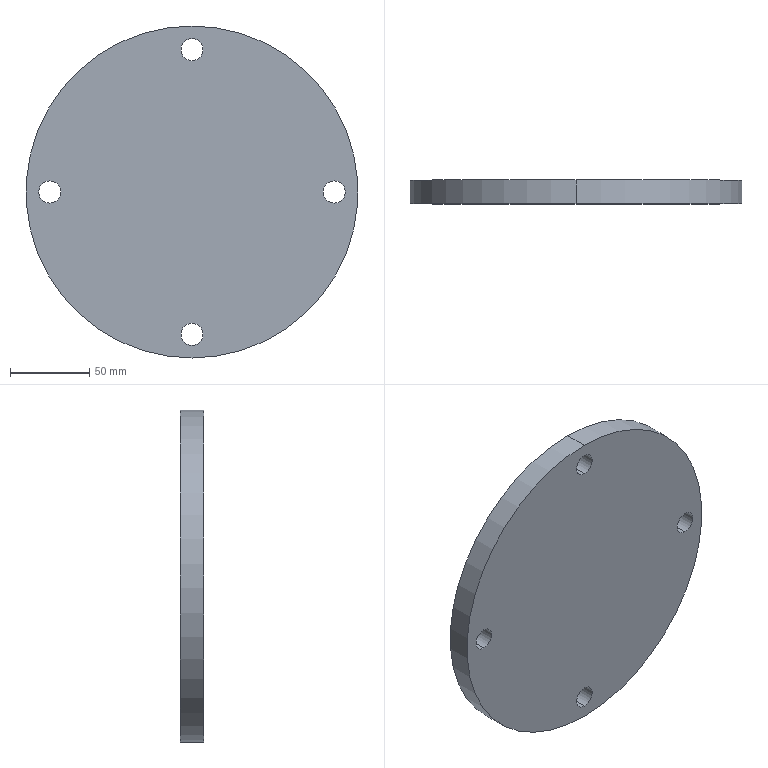Part | SolidWorks | features Extrusion 1, HoleWzd 1, RefAxis 1 | 1 solid | 12 faces | box 210 x 15 x 210 mm | volume 510305 mm3 | cylinder 10 | plane 2 | commonest cylinder face diameters 14 x8 210 x2
STEP:
#1=CARTESIAN_POINT('',(0.,0.,-97.));
#2=VERTEX_POINT('',#1);
#3=CARTESIAN_POINT('',(0.,0.,-83.));
#4=VERTEX_POINT('',#3);
#5=CARTESIAN_POINT('',(0.,0.,-90.));
#6=DIRECTION('',(0.,1.,0.));
#7=DIRECTION('',(0.,0.,1.));
#8=AXIS2_PLACEMENT_3D('',#5,#6,#7);
#9=CIRCLE('',#8,7.);
#10=EDGE_CURVE('',#2,#4,#9,.T.);
#11=ORIENTED_EDGE('',*,*,#10,.F.);
#12=CARTESIAN_POINT('',(0.,15.,-97.));
#13=VERTEX_POINT('',#12);
#14=CARTESIAN_POINT('',(0.,15.,-97.));
#15=DIRECTION('',(0.,1.,0.));
#16=VECTOR('',#15,1000.);
#17=LINE('',#14,#16);
#18=EDGE_CURVE('',#2,#13,#17,.T.);
#19=ORIENTED_EDGE('',*,*,#18,.T.);
#20=CARTESIAN_POINT('',(0.,15.,-83.));
#21=VERTEX_POINT('',#20);
#22=CARTESIAN_POINT('',(0.,15.,-90.));
#23=DIRECTION('',(0.,1.,0.));
#24=DIRECTION('',(0.,0.,1.));
#25=AXIS2_PLACEMENT_3D('',#22,#23,#24);
#26=CIRCLE('',#25,7.);
#27=EDGE_CURVE('',#13,#21,#26,.T.);
#28=ORIENTED_EDGE('',*,*,#27,.T.);
#29=CARTESIAN_POINT('',(0.,15.,-83.));
#30=DIRECTION('',(0.,1.,0.));
#31=VECTOR('',#30,1000.);
#32=LINE('',#29,#31);
#33=EDGE_CURVE('',#4,#21,#32,.T.);
#34=ORIENTED_EDGE('',*,*,#33,.F.);
#35=EDGE_LOOP('',(#11,#19,#28,#34));
#36=FACE_OUTER_BOUND('',#35,.T.);
#37=CARTESIAN_POINT('',(0.,15.,-90.));
#38=DIRECTION('',(0.,1.,0.));
#39=DIRECTION('',(0.,0.,1.));
#40=AXIS2_PLACEMENT_3D('',#37,#38,#39);
#41=CYLINDRICAL_SURFACE('',#40,7.);
#42=ADVANCED_FACE('',(#36),#41,.F.);
#43=CARTESIAN_POINT('',(90.,0.,-7.));
#44=VERTEX_POINT('',#43);
#45=CARTESIAN_POINT('',(90.,0.,7.));
#46=VERTEX_POINT('',#45);
#47=CARTESIAN_POINT('',(90.,0.,0.));
#48=DIRECTION('',(0.,1.,0.));
#49=DIRECTION('',(0.,0.,1.));
#50=AXIS2_PLACEMENT_3D('',#47,#48,#49);
#51=CIRCLE('',#50,7.);
#52=EDGE_CURVE('',#44,#46,#51,.T.);
#53=ORIENTED_EDGE('',*,*,#52,.F.);
#54=CARTESIAN_POINT('',(90.,15.,-7.));
#55=VERTEX_POINT('',#54);
#56=CARTESIAN_POINT('',(90.,15.,-7.));
#57=DIRECTION('',(0.,1.,0.));
#58=VECTOR('',#57,1000.);
#59=LINE('',#56,#58);
#60=EDGE_CURVE('',#44,#55,#59,.T.);
#61=ORIENTED_EDGE('',*,*,#60,.T.);
#62=CARTESIAN_POINT('',(90.,15.,7.));
#63=VERTEX_POINT('',#62);
#64=CARTESIAN_POINT('',(90.,15.,0.));
#65=DIRECTION('',(0.,1.,0.));
#66=DIRECTION('',(0.,0.,1.));
#67=AXIS2_PLACEMENT_3D('',#64,#65,#66);
#68=CIRCLE('',#67,7.);
#69=EDGE_CURVE('',#55,#63,#68,.T.);
#70=ORIENTED_EDGE('',*,*,#69,.T.);
#71=CARTESIAN_POINT('',(90.,15.,7.));
#72=DIRECTION('',(0.,1.,0.));
#73=VECTOR('',#72,1000.);
#74=LINE('',#71,#73);
#75=EDGE_CURVE('',#46,#63,#74,.T.);
#76=ORIENTED_EDGE('',*,*,#75,.F.);
#77=EDGE_LOOP('',(#53,#61,#70,#76));
#78=FACE_OUTER_BOUND('',#77,.T.);
#79=CARTESIAN_POINT('',(90.,15.,0.));
#80=DIRECTION('',(0.,1.,0.));
#81=DIRECTION('',(0.,0.,1.));
#82=AXIS2_PLACEMENT_3D('',#79,#80,#81);
#83=CYLINDRICAL_SURFACE('',#82,7.);
#84=ADVANCED_FACE('',(#78),#83,.F.);
#85=CARTESIAN_POINT('',(0.,0.,83.));
#86=VERTEX_POINT('',#85);
#87=CARTESIAN_POINT('',(0.,0.,97.));
#88=VERTEX_POINT('',#87);
#89=CARTESIAN_POINT('',(0.,0.,90.));
#90=DIRECTION('',(0.,1.,0.));
#91=DIRECTION('',(0.,0.,1.));
#92=AXIS2_PLACEMENT_3D('',#89,#90,#91);
#93=CIRCLE('',#92,7.);
#94=EDGE_CURVE('',#86,#88,#93,.T.);
#95=ORIENTED_EDGE('',*,*,#94,.F.);
#96=CARTESIAN_POINT('',(0.,15.,83.));
#97=VERTEX_POINT('',#96);
#98=CARTESIAN_POINT('',(0.,15.,83.));
#99=DIRECTION('',(0.,1.,0.));
#100=VECTOR('',#99,1000.);
#101=LINE('',#98,#100);
#102=EDGE_CURVE('',#86,#97,#101,.T.);
#103=ORIENTED_EDGE('',*,*,#102,.T.);
#104=CARTESIAN_POINT('',(0.,15.,97.));
#105=VERTEX_POINT('',#104);
#106=CARTESIAN_POINT('',(0.,15.,90.));
#107=DIRECTION('',(0.,1.,0.));
#108=DIRECTION('',(0.,0.,1.));
#109=AXIS2_PLACEMENT_3D('',#106,#107,#108);
#110=CIRCLE('',#109,7.);
#111=EDGE_CURVE('',#97,#105,#110,.T.);
#112=ORIENTED_EDGE('',*,*,#111,.T.);
#113=CARTESIAN_POINT('',(0.,15.,97.));
#114=DIRECTION('',(0.,1.,0.));
#115=VECTOR('',#114,1000.);
#116=LINE('',#113,#115);
#117=EDGE_CURVE('',#88,#105,#116,.T.);
#118=ORIENTED_EDGE('',*,*,#117,.F.);
#119=EDGE_LOOP('',(#95,#103,#112,#118));
#120=FACE_OUTER_BOUND('',#119,.T.);
#121=CARTESIAN_POINT('',(0.,15.,90.));
#122=DIRECTION('',(0.,1.,0.));
#123=DIRECTION('',(0.,0.,1.));
#124=AXIS2_PLACEMENT_3D('',#121,#122,#123);
#125=CYLINDRICAL_SURFACE('',#124,7.);
#126=ADVANCED_FACE('',(#120),#125,.F.);
#127=CARTESIAN_POINT('',(-90.,0.,-7.));
#128=VERTEX_POINT('',#127);
#129=CARTESIAN_POINT('',(-90.,0.,7.));
#130=VERTEX_POINT('',#129);
#131=CARTESIAN_POINT('',(-90.,0.,0.));
#132=DIRECTION('',(0.,1.,0.));
#133=DIRECTION('',(0.,0.,1.));
#134=AXIS2_PLACEMENT_3D('',#131,#132,#133);
#135=CIRCLE('',#134,7.);
#136=EDGE_CURVE('',#128,#130,#135,.T.);
#137=ORIENTED_EDGE('',*,*,#136,.F.);
#138=CARTESIAN_POINT('',(-90.,15.,-7.));
#139=VERTEX_POINT('',#138);
#140=CARTESIAN_POINT('',(-90.,15.,-7.));
#141=DIRECTION('',(0.,1.,0.));
#142=VECTOR('',#141,1000.);
#143=LINE('',#140,#142);
#144=EDGE_CURVE('',#128,#139,#143,.T.);
#145=ORIENTED_EDGE('',*,*,#144,.T.);
#146=CARTESIAN_POINT('',(-90.,15.,7.));
#147=VERTEX_POINT('',#146);
#148=CARTESIAN_POINT('',(-90.,15.,0.));
#149=DIRECTION('',(0.,1.,0.));
#150=DIRECTION('',(0.,0.,1.));
#151=AXIS2_PLACEMENT_3D('',#148,#149,#150);
#152=CIRCLE('',#151,7.);
#153=EDGE_CURVE('',#139,#147,#152,.T.);
#154=ORIENTED_EDGE('',*,*,#153,.T.);
#155=CARTESIAN_POINT('',(-90.,15.,7.));
#156=DIRECTION('',(0.,1.,0.));
#157=VECTOR('',#156,1000.);
#158=LINE('',#155,#157);
#159=EDGE_CURVE('',#130,#147,#158,.T.);
#160=ORIENTED_EDGE('',*,*,#159,.F.);
#161=EDGE_LOOP('',(#137,#145,#154,#160));
#162=FACE_OUTER_BOUND('',#161,.T.);
#163=CARTESIAN_POINT('',(-90.,15.,0.));
#164=DIRECTION('',(0.,1.,0.));
#165=DIRECTION('',(0.,0.,1.));
#166=AXIS2_PLACEMENT_3D('',#163,#164,#165);
#167=CYLINDRICAL_SURFACE('',#166,7.);
#168=ADVANCED_FACE('',(#162),#167,.F.);
#169=CARTESIAN_POINT('',(0.,15.,105.));
#170=VERTEX_POINT('',#169);
#171=CARTESIAN_POINT('',(0.,15.,-105.));
#172=VERTEX_POINT('',#171);
#173=CARTESIAN_POINT('',(0.,15.,0.));
#174=DIRECTION('',(0.,1.,0.));
#175=DIRECTION('',(0.,0.,1.));
#176=AXIS2_PLACEMENT_3D('',#173,#174,#175);
#177=CIRCLE('',#176,105.);
#178=EDGE_CURVE('',#170,#172,#177,.T.);
#179=ORIENTED_EDGE('',*,*,#178,.F.);
#180=CARTESIAN_POINT('',(0.,0.,105.));
#181=VERTEX_POINT('',#180);
#182=CARTESIAN_POINT('',(0.,15.,105.));
#183=DIRECTION('',(0.,-1.,0.));
#184=VECTOR('',#183,1000.);
#185=LINE('',#182,#184);
#186=EDGE_CURVE('',#170,#181,#185,.T.);
#187=ORIENTED_EDGE('',*,*,#186,.T.);
#188=CARTESIAN_POINT('',(0.,0.,-105.));
#189=VERTEX_POINT('',#188);
#190=CARTESIAN_POINT('',(0.,0.,0.));
#191=DIRECTION('',(0.,1.,0.));
#192=DIRECTION('',(0.,0.,1.));
#193=AXIS2_PLACEMENT_3D('',#190,#191,#192);
#194=CIRCLE('',#193,105.);
#195=EDGE_CURVE('',#181,#189,#194,.T.);
#196=ORIENTED_EDGE('',*,*,#195,.T.);
#197=CARTESIAN_POINT('',(0.,15.,-105.));
#198=DIRECTION('',(0.,-1.,0.));
#199=VECTOR('',#198,1000.);
#200=LINE('',#197,#199);
#201=EDGE_CURVE('',#172,#189,#200,.T.);
#202=ORIENTED_EDGE('',*,*,#201,.F.);
#203=EDGE_LOOP('',(#179,#187,#196,#202));
#204=FACE_OUTER_BOUND('',#203,.T.);
#205=CARTESIAN_POINT('',(0.,15.,0.));
#206=DIRECTION('',(0.,-1.,0.));
#207=DIRECTION('',(0.,0.,-1.));
#208=AXIS2_PLACEMENT_3D('',#205,#206,#207);
#209=CYLINDRICAL_SURFACE('',#208,105.);
#210=ADVANCED_FACE('',(#204),#209,.T.);
#211=ORIENTED_EDGE('',*,*,#186,.F.);
#212=CARTESIAN_POINT('',(0.,15.,0.));
#213=DIRECTION('',(0.,1.,0.));
#214=DIRECTION('',(0.,0.,1.));
#215=AXIS2_PLACEMENT_3D('',#212,#213,#214);
#216=CIRCLE('',#215,105.);
#217=EDGE_CURVE('',#172,#170,#216,.T.);
#218=ORIENTED_EDGE('',*,*,#217,.F.);
#219=ORIENTED_EDGE('',*,*,#201,.T.);
#220=CARTESIAN_POINT('',(0.,0.,0.));
#221=DIRECTION('',(0.,1.,0.));
#222=DIRECTION('',(0.,0.,1.));
#223=AXIS2_PLACEMENT_3D('',#220,#221,#222);
#224=CIRCLE('',#223,105.);
#225=EDGE_CURVE('',#189,#181,#224,.T.);
#226=ORIENTED_EDGE('',*,*,#225,.T.);
#227=EDGE_LOOP('',(#211,#218,#219,#226));
#228=FACE_OUTER_BOUND('',#227,.T.);
#229=CARTESIAN_POINT('',(0.,15.,0.));
#230=DIRECTION('',(0.,-1.,0.));
#231=DIRECTION('',(0.,0.,-1.));
#232=AXIS2_PLACEMENT_3D('',#229,#230,#231);
#233=CYLINDRICAL_SURFACE('',#232,105.);
#234=ADVANCED_FACE('',(#228),#233,.T.);
#235=CARTESIAN_POINT('',(0.,15.,-90.));
#236=DIRECTION('',(0.,1.,0.));
#237=DIRECTION('',(0.,0.,1.));
#238=AXIS2_PLACEMENT_3D('',#235,#236,#237);
#239=CIRCLE('',#238,7.);
#240=EDGE_CURVE('',#21,#13,#239,.T.);
#241=ORIENTED_EDGE('',*,*,#240,.F.);
#242=ORIENTED_EDGE('',*,*,#27,.F.);
#243=EDGE_LOOP('',(#241,#242));
#244=FACE_BOUND('',#243,.T.);
#245=CARTESIAN_POINT('',(90.,15.,0.));
#246=DIRECTION('',(0.,1.,0.));
#247=DIRECTION('',(0.,0.,1.));
#248=AXIS2_PLACEMENT_3D('',#245,#246,#247);
#249=CIRCLE('',#248,7.);
#250=EDGE_CURVE('',#63,#55,#249,.T.);
#251=ORIENTED_EDGE('',*,*,#250,.F.);
#252=ORIENTED_EDGE('',*,*,#69,.F.);
#253=EDGE_LOOP('',(#251,#252));
#254=FACE_BOUND('',#253,.T.);
#255=CARTESIAN_POINT('',(0.,15.,90.));
#256=DIRECTION('',(0.,1.,0.));
#257=DIRECTION('',(0.,0.,1.));
#258=AXIS2_PLACEMENT_3D('',#255,#256,#257);
#259=CIRCLE('',#258,7.);
#260=EDGE_CURVE('',#105,#97,#259,.T.);
#261=ORIENTED_EDGE('',*,*,#260,.F.);
#262=ORIENTED_EDGE('',*,*,#111,.F.);
#263=EDGE_LOOP('',(#261,#262));
#264=FACE_BOUND('',#263,.T.);
#265=CARTESIAN_POINT('',(-90.,15.,0.));
#266=DIRECTION('',(0.,1.,0.));
#267=DIRECTION('',(0.,0.,1.));
#268=AXIS2_PLACEMENT_3D('',#265,#266,#267);
#269=CIRCLE('',#268,7.);
#270=EDGE_CURVE('',#147,#139,#269,.T.);
#271=ORIENTED_EDGE('',*,*,#270,.F.);
#272=ORIENTED_EDGE('',*,*,#153,.F.);
#273=EDGE_LOOP('',(#271,#272));
#274=FACE_BOUND('',#273,.T.);
#275=ORIENTED_EDGE('',*,*,#217,.T.);
#276=ORIENTED_EDGE('',*,*,#178,.T.);
#277=EDGE_LOOP('',(#275,#276));
#278=FACE_OUTER_BOUND('',#277,.T.);
#279=CARTESIAN_POINT('',(0.,15.,0.));
#280=DIRECTION('',(0.,1.,0.));
#281=DIRECTION('',(0.,0.,1.));
#282=AXIS2_PLACEMENT_3D('',#279,#280,#281);
#283=PLANE('',#282);
#284=ADVANCED_FACE('',(#244,#254,#264,#274,#278),#283,.T.);
#285=CARTESIAN_POINT('',(0.,0.,-90.));
#286=DIRECTION('',(0.,1.,0.));
#287=DIRECTION('',(0.,0.,1.));
#288=AXIS2_PLACEMENT_3D('',#285,#286,#287);
#289=CIRCLE('',#288,7.);
#290=EDGE_CURVE('',#4,#2,#289,.T.);
#291=ORIENTED_EDGE('',*,*,#290,.T.);
#292=ORIENTED_EDGE('',*,*,#10,.T.);
#293=EDGE_LOOP('',(#291,#292));
#294=FACE_BOUND('',#293,.T.);
#295=CARTESIAN_POINT('',(90.,0.,0.));
#296=DIRECTION('',(0.,1.,0.));
#297=DIRECTION('',(0.,0.,1.));
#298=AXIS2_PLACEMENT_3D('',#295,#296,#297);
#299=CIRCLE('',#298,7.);
#300=EDGE_CURVE('',#46,#44,#299,.T.);
#301=ORIENTED_EDGE('',*,*,#300,.T.);
#302=ORIENTED_EDGE('',*,*,#52,.T.);
#303=EDGE_LOOP('',(#301,#302));
#304=FACE_BOUND('',#303,.T.);
#305=CARTESIAN_POINT('',(0.,0.,90.));
#306=DIRECTION('',(0.,1.,0.));
#307=DIRECTION('',(0.,0.,1.));
#308=AXIS2_PLACEMENT_3D('',#305,#306,#307);
#309=CIRCLE('',#308,7.);
#310=EDGE_CURVE('',#88,#86,#309,.T.);
#311=ORIENTED_EDGE('',*,*,#310,.T.);
#312=ORIENTED_EDGE('',*,*,#94,.T.);
#313=EDGE_LOOP('',(#311,#312));
#314=FACE_BOUND('',#313,.T.);
#315=CARTESIAN_POINT('',(-90.,0.,0.));
#316=DIRECTION('',(0.,1.,0.));
#317=DIRECTION('',(0.,0.,1.));
#318=AXIS2_PLACEMENT_3D('',#315,#316,#317);
#319=CIRCLE('',#318,7.);
#320=EDGE_CURVE('',#130,#128,#319,.T.);
#321=ORIENTED_EDGE('',*,*,#320,.T.);
#322=ORIENTED_EDGE('',*,*,#136,.T.);
#323=EDGE_LOOP('',(#321,#322));
#324=FACE_BOUND('',#323,.T.);
#325=ORIENTED_EDGE('',*,*,#225,.F.);
#326=ORIENTED_EDGE('',*,*,#195,.F.);
#327=EDGE_LOOP('',(#325,#326));
#328=FACE_OUTER_BOUND('',#327,.T.);
#329=CARTESIAN_POINT('',(0.,0.,0.));
#330=DIRECTION('',(0.,1.,0.));
#331=DIRECTION('',(0.,0.,1.));
#332=AXIS2_PLACEMENT_3D('',#329,#330,#331);
#333=PLANE('',#332);
#334=ADVANCED_FACE('',(#294,#304,#314,#324,#328),#333,.F.);
#335=ORIENTED_EDGE('',*,*,#144,.F.);
#336=ORIENTED_EDGE('',*,*,#320,.F.);
#337=ORIENTED_EDGE('',*,*,#159,.T.);
#338=ORIENTED_EDGE('',*,*,#270,.T.);
#339=EDGE_LOOP('',(#335,#336,#337,#338));
#340=FACE_OUTER_BOUND('',#339,.T.);
#341=CARTESIAN_POINT('',(-90.,15.,0.));
#342=DIRECTION('',(0.,1.,0.));
#343=DIRECTION('',(0.,0.,1.));
#344=AXIS2_PLACEMENT_3D('',#341,#342,#343);
#345=CYLINDRICAL_SURFACE('',#344,7.);
#346=ADVANCED_FACE('',(#340),#345,.F.);
#347=ORIENTED_EDGE('',*,*,#102,.F.);
#348=ORIENTED_EDGE('',*,*,#310,.F.);
#349=ORIENTED_EDGE('',*,*,#117,.T.);
#350=ORIENTED_EDGE('',*,*,#260,.T.);
#351=EDGE_LOOP('',(#347,#348,#349,#350));
#352=FACE_OUTER_BOUND('',#351,.T.);
#353=CARTESIAN_POINT('',(0.,15.,90.));
#354=DIRECTION('',(0.,1.,0.));
#355=DIRECTION('',(0.,0.,1.));
#356=AXIS2_PLACEMENT_3D('',#353,#354,#355);
#357=CYLINDRICAL_SURFACE('',#356,7.);
#358=ADVANCED_FACE('',(#352),#357,.F.);
#359=ORIENTED_EDGE('',*,*,#60,.F.);
#360=ORIENTED_EDGE('',*,*,#300,.F.);
#361=ORIENTED_EDGE('',*,*,#75,.T.);
#362=ORIENTED_EDGE('',*,*,#250,.T.);
#363=EDGE_LOOP('',(#359,#360,#361,#362));
#364=FACE_OUTER_BOUND('',#363,.T.);
#365=CARTESIAN_POINT('',(90.,15.,0.));
#366=DIRECTION('',(0.,1.,0.));
#367=DIRECTION('',(0.,0.,1.));
#368=AXIS2_PLACEMENT_3D('',#365,#366,#367);
#369=CYLINDRICAL_SURFACE('',#368,7.);
#370=ADVANCED_FACE('',(#364),#369,.F.);
#371=ORIENTED_EDGE('',*,*,#18,.F.);
#372=ORIENTED_EDGE('',*,*,#290,.F.);
#373=ORIENTED_EDGE('',*,*,#33,.T.);
#374=ORIENTED_EDGE('',*,*,#240,.T.);
#375=EDGE_LOOP('',(#371,#372,#373,#374));
#376=FACE_OUTER_BOUND('',#375,.T.);
#377=CARTESIAN_POINT('',(0.,15.,-90.));
#378=DIRECTION('',(0.,1.,0.));
#379=DIRECTION('',(0.,0.,1.));
#380=AXIS2_PLACEMENT_3D('',#377,#378,#379);
#381=CYLINDRICAL_SURFACE('',#380,7.);
#382=ADVANCED_FACE('',(#376),#381,.F.);
#383=CLOSED_SHELL('',(#42,#84,#126,#168,#210,#234,#284,#334,#346,#358,#370,#382));
#384=MANIFOLD_SOLID_BREP('',#383);
#385=CARTESIAN_POINT('',(0.,0.,0.));
#386=DIRECTION('',(0.,0.,1.));
#387=DIRECTION('',(1.,0.,0.));
#388=AXIS2_PLACEMENT_3D('',#385,#386,#387);
#389=(LENGTH_UNIT()NAMED_UNIT(*)SI_UNIT(.MILLI.,.METRE.));
#390=UNCERTAINTY_MEASURE_WITH_UNIT(LENGTH_MEASURE(0.00001),#389,'','');
#391=(NAMED_UNIT(*)PLANE_ANGLE_UNIT()SI_UNIT($,.RADIAN.));
#392=(NAMED_UNIT(*)SI_UNIT($,.STERADIAN.)SOLID_ANGLE_UNIT());
#393=(GEOMETRIC_REPRESENTATION_CONTEXT(3)GLOBAL_UNCERTAINTY_ASSIGNED_CONTEXT((#390))GLOBAL_UNIT_ASSIGNED_CONTEXT((#389,#391,#392))REPRESENTATION_CONTEXT('',''));
#394=ADVANCED_BREP_SHAPE_REPRESENTATION('',(#384,#388),#393);